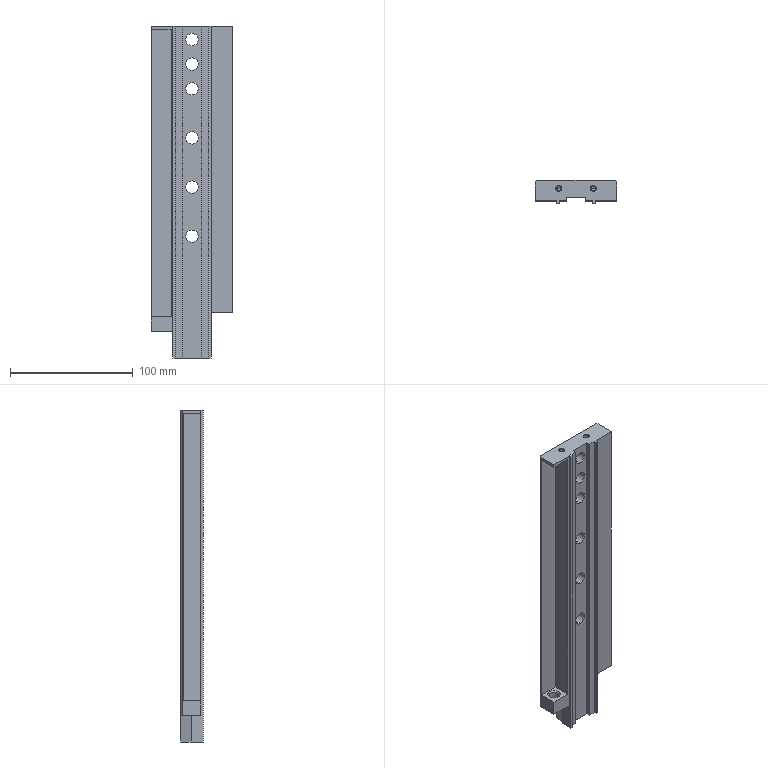Part | STEP file | 1 solid | 104 faces | box 66 x 18.5 x 270 mm | volume 203255 mm3 | plane 38 | cylinder 37 | cone 29 | commonest cylinder face diameters 4 x16 10 x14 5 x5 8 x2